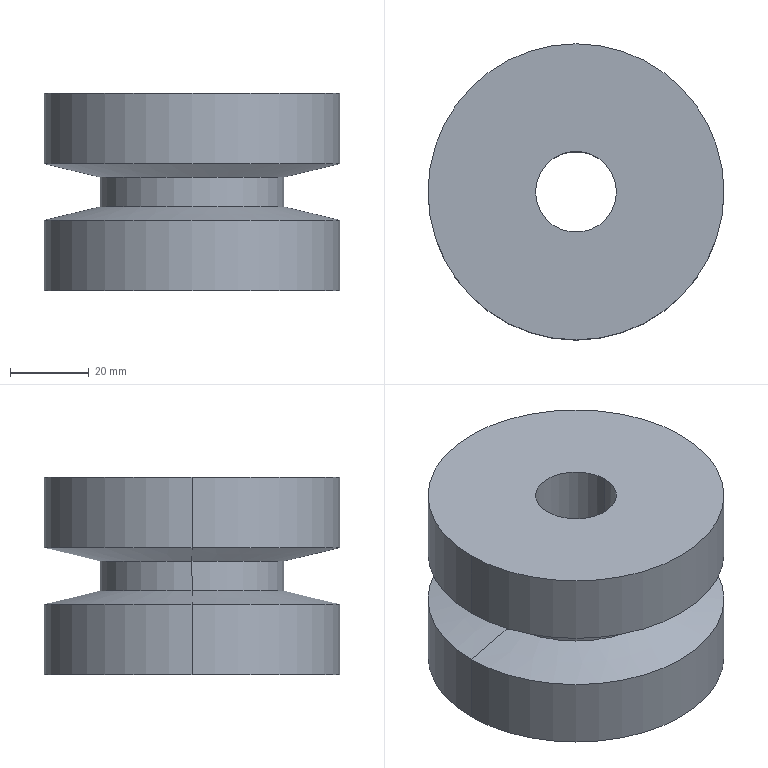Part | SolidWorks | features HoleWzd 2, Extrusion 1, RevCut 1 | 1 solid | 20 faces | box 75 x 75 x 50 mm | volume 173343 mm3 | cylinder 12 | cone 4 | plane 4 | commonest cylinder face diameters 4.2 x4 75 x4 20.5 x2 46.5 x2
STEP:
#1=CARTESIAN_POINT('',(10.25,0.,6.9));
#2=VERTEX_POINT('',#1);
#3=CARTESIAN_POINT('',(10.25,0.,11.1));
#4=VERTEX_POINT('',#3);
#5=CARTESIAN_POINT('',(10.25,0.,6.9));
#6=CARTESIAN_POINT('',(10.25,-0.1391,6.9));
#7=CARTESIAN_POINT('',(10.247,-0.2759,6.914));
#8=CARTESIAN_POINT('',(10.236,-0.5448,6.967));
#9=CARTESIAN_POINT('',(10.228,-0.6784,7.008));
#10=CARTESIAN_POINT('',(10.208,-0.9326,7.113));
#11=CARTESIAN_POINT('',(10.196,-1.053,7.178));
#12=CARTESIAN_POINT('',(10.17,-1.281,7.33));
#13=CARTESIAN_POINT('',(10.156,-1.389,7.419));
#14=CARTESIAN_POINT('',(10.114,-1.678,7.709));
#15=CARTESIAN_POINT('',(10.085,-1.835,7.942));
#16=CARTESIAN_POINT('',(10.055,-1.992,8.321));
#17=CARTESIAN_POINT('',(10.047,-2.032,8.454));
#18=CARTESIAN_POINT('',(10.035,-2.087,8.725));
#19=CARTESIAN_POINT('',(10.033,-2.1,8.862));
#20=CARTESIAN_POINT('',(10.033,-2.1,9.137));
#21=CARTESIAN_POINT('',(10.035,-2.086,9.276));
#22=CARTESIAN_POINT('',(10.047,-2.032,9.546));
#23=CARTESIAN_POINT('',(10.055,-1.993,9.677));
#24=CARTESIAN_POINT('',(10.085,-1.834,10.059));
#25=CARTESIAN_POINT('',(10.113,-1.68,10.29));
#26=CARTESIAN_POINT('',(10.156,-1.387,10.583));
#27=CARTESIAN_POINT('',(10.17,-1.282,10.669));
#28=CARTESIAN_POINT('',(10.196,-1.054,10.821));
#29=CARTESIAN_POINT('',(10.208,-0.9314,10.887));
#30=CARTESIAN_POINT('',(10.228,-0.6776,10.992));
#31=CARTESIAN_POINT('',(10.236,-0.5466,11.032));
#32=CARTESIAN_POINT('',(10.247,-0.2767,11.086));
#33=CARTESIAN_POINT('',(10.25,-0.1373,11.1));
#34=CARTESIAN_POINT('',(10.25,0.,11.1));
#35=B_SPLINE_CURVE_WITH_KNOTS('',3,(#5,#6,#7,#8,#9,#10,#11,#12,#13,#14,#15,#16,#17,#18,#19,#20,#21,#22,#23,#24,#25,#26,#27,#28,#29,#30,#31,#32,#33,#34),.UNSPECIFIED.,.F.,.F.,(4,2,2,2,2,2,2,2,2,2,2,2,2,2,4),(0.,0.0004114,0.0008229,0.001234,0.001646,0.002469,0.00288,0.003292,0.003703,0.004114,0.004937,0.005349,0.00576,0.006172,0.006583),.UNSPECIFIED.);
#36=EDGE_CURVE('',#2,#4,#35,.T.);
#37=ORIENTED_EDGE('',*,*,#36,.T.);
#38=CARTESIAN_POINT('',(32.5,0.,11.1));
#39=VERTEX_POINT('',#38);
#40=CARTESIAN_POINT('',(32.5,0.,11.1));
#41=DIRECTION('',(1.,0.,0.));
#42=VECTOR('',#41,1000.);
#43=LINE('',#40,#42);
#44=EDGE_CURVE('',#4,#39,#43,.T.);
#45=ORIENTED_EDGE('',*,*,#44,.T.);
#46=CARTESIAN_POINT('',(32.5,0.,6.9));
#47=VERTEX_POINT('',#46);
#48=CARTESIAN_POINT('',(32.5,0.,9.));
#49=DIRECTION('',(1.,0.,0.));
#50=DIRECTION('',(0.,0.,-1.));
#51=AXIS2_PLACEMENT_3D('',#48,#49,#50);
#52=CIRCLE('',#51,2.1);
#53=EDGE_CURVE('',#39,#47,#52,.T.);
#54=ORIENTED_EDGE('',*,*,#53,.T.);
#55=CARTESIAN_POINT('',(32.5,0.,6.9));
#56=DIRECTION('',(1.,0.,0.));
#57=VECTOR('',#56,1000.);
#58=LINE('',#55,#57);
#59=EDGE_CURVE('',#2,#47,#58,.T.);
#60=ORIENTED_EDGE('',*,*,#59,.F.);
#61=EDGE_LOOP('',(#37,#45,#54,#60));
#62=FACE_OUTER_BOUND('',#61,.T.);
#63=CARTESIAN_POINT('',(32.5,0.,9.));
#64=DIRECTION('',(1.,0.,0.));
#65=DIRECTION('',(0.,0.,-1.));
#66=AXIS2_PLACEMENT_3D('',#63,#64,#65);
#67=CYLINDRICAL_SURFACE('',#66,2.1);
#68=ADVANCED_FACE('',(#62),#67,.F.);
#69=CARTESIAN_POINT('',(0.,10.25,11.1));
#70=VERTEX_POINT('',#69);
#71=CARTESIAN_POINT('',(0.,10.25,6.9));
#72=VERTEX_POINT('',#71);
#73=CARTESIAN_POINT('',(0.,10.25,11.1));
#74=CARTESIAN_POINT('',(-0.1391,10.25,11.1));
#75=CARTESIAN_POINT('',(-0.2759,10.247,11.086));
#76=CARTESIAN_POINT('',(-0.5448,10.236,11.033));
#77=CARTESIAN_POINT('',(-0.6784,10.228,10.992));
#78=CARTESIAN_POINT('',(-0.9326,10.208,10.887));
#79=CARTESIAN_POINT('',(-1.053,10.196,10.822));
#80=CARTESIAN_POINT('',(-1.281,10.17,10.67));
#81=CARTESIAN_POINT('',(-1.389,10.156,10.581));
#82=CARTESIAN_POINT('',(-1.678,10.114,10.291));
#83=CARTESIAN_POINT('',(-1.835,10.085,10.058));
#84=CARTESIAN_POINT('',(-1.992,10.055,9.679));
#85=CARTESIAN_POINT('',(-2.032,10.047,9.546));
#86=CARTESIAN_POINT('',(-2.087,10.035,9.275));
#87=CARTESIAN_POINT('',(-2.1,10.033,9.138));
#88=CARTESIAN_POINT('',(-2.1,10.033,8.863));
#89=CARTESIAN_POINT('',(-2.086,10.035,8.724));
#90=CARTESIAN_POINT('',(-2.032,10.047,8.454));
#91=CARTESIAN_POINT('',(-1.993,10.055,8.323));
#92=CARTESIAN_POINT('',(-1.834,10.085,7.941));
#93=CARTESIAN_POINT('',(-1.68,10.113,7.71));
#94=CARTESIAN_POINT('',(-1.387,10.156,7.417));
#95=CARTESIAN_POINT('',(-1.282,10.17,7.331));
#96=CARTESIAN_POINT('',(-1.054,10.196,7.179));
#97=CARTESIAN_POINT('',(-0.9314,10.208,7.113));
#98=CARTESIAN_POINT('',(-0.6776,10.228,7.008));
#99=CARTESIAN_POINT('',(-0.5466,10.236,6.968));
#100=CARTESIAN_POINT('',(-0.2767,10.247,6.914));
#101=CARTESIAN_POINT('',(-0.1373,10.25,6.9));
#102=CARTESIAN_POINT('',(0.,10.25,6.9));
#103=B_SPLINE_CURVE_WITH_KNOTS('',3,(#73,#74,#75,#76,#77,#78,#79,#80,#81,#82,#83,#84,#85,#86,#87,#88,#89,#90,#91,#92,#93,#94,#95,#96,#97,#98,#99,#100,#101,#102),.UNSPECIFIED.,.F.,.F.,(4,2,2,2,2,2,2,2,2,2,2,2,2,2,4),(0.,0.0004114,0.0008229,0.001234,0.001646,0.002469,0.00288,0.003292,0.003703,0.004114,0.004937,0.005349,0.00576,0.006172,0.006583),.UNSPECIFIED.);
#104=EDGE_CURVE('',#70,#72,#103,.T.);
#105=ORIENTED_EDGE('',*,*,#104,.T.);
#106=CARTESIAN_POINT('',(0.,32.5,6.9));
#107=VERTEX_POINT('',#106);
#108=CARTESIAN_POINT('',(0.,32.5,6.9));
#109=DIRECTION('',(0.,1.,0.));
#110=VECTOR('',#109,1000.);
#111=LINE('',#108,#110);
#112=EDGE_CURVE('',#72,#107,#111,.T.);
#113=ORIENTED_EDGE('',*,*,#112,.T.);
#114=CARTESIAN_POINT('',(0.,32.5,11.1));
#115=VERTEX_POINT('',#114);
#116=CARTESIAN_POINT('',(0.,32.5,9.));
#117=DIRECTION('',(0.,1.,0.));
#118=DIRECTION('',(0.,0.,1.));
#119=AXIS2_PLACEMENT_3D('',#116,#117,#118);
#120=CIRCLE('',#119,2.1);
#121=EDGE_CURVE('',#107,#115,#120,.T.);
#122=ORIENTED_EDGE('',*,*,#121,.T.);
#123=CARTESIAN_POINT('',(0.,32.5,11.1));
#124=DIRECTION('',(0.,1.,0.));
#125=VECTOR('',#124,1000.);
#126=LINE('',#123,#125);
#127=EDGE_CURVE('',#70,#115,#126,.T.);
#128=ORIENTED_EDGE('',*,*,#127,.F.);
#129=EDGE_LOOP('',(#105,#113,#122,#128));
#130=FACE_OUTER_BOUND('',#129,.T.);
#131=CARTESIAN_POINT('',(0.,32.5,9.));
#132=DIRECTION('',(0.,1.,0.));
#133=DIRECTION('',(0.,0.,1.));
#134=AXIS2_PLACEMENT_3D('',#131,#132,#133);
#135=CYLINDRICAL_SURFACE('',#134,2.1);
#136=ADVANCED_FACE('',(#130),#135,.F.);
#137=CARTESIAN_POINT('',(-23.25,0.,28.75));
#138=VERTEX_POINT('',#137);
#139=CARTESIAN_POINT('',(23.25,0.,28.75));
#140=VERTEX_POINT('',#139);
#141=CARTESIAN_POINT('',(0.,0.,28.75));
#142=DIRECTION('',(0.,0.,-1.));
#143=DIRECTION('',(-1.,0.,0.));
#144=AXIS2_PLACEMENT_3D('',#141,#142,#143);
#145=CIRCLE('',#144,23.25);
#146=EDGE_CURVE('',#138,#140,#145,.T.);
#147=ORIENTED_EDGE('',*,*,#146,.T.);
#148=CARTESIAN_POINT('',(23.25,0.,21.25));
#149=VERTEX_POINT('',#148);
#150=CARTESIAN_POINT('',(23.25,0.,0.));
#151=DIRECTION('',(0.,0.,-1.));
#152=VECTOR('',#151,1000.);
#153=LINE('',#150,#152);
#154=EDGE_CURVE('',#140,#149,#153,.T.);
#155=ORIENTED_EDGE('',*,*,#154,.T.);
#156=CARTESIAN_POINT('',(-23.25,0.,21.25));
#157=VERTEX_POINT('',#156);
#158=CARTESIAN_POINT('',(0.,0.,21.25));
#159=DIRECTION('',(0.,0.,-1.));
#160=DIRECTION('',(-1.,0.,0.));
#161=AXIS2_PLACEMENT_3D('',#158,#159,#160);
#162=CIRCLE('',#161,23.25);
#163=EDGE_CURVE('',#157,#149,#162,.T.);
#164=ORIENTED_EDGE('',*,*,#163,.F.);
#165=CARTESIAN_POINT('',(-23.25,0.,0.));
#166=DIRECTION('',(0.,0.,-1.));
#167=VECTOR('',#166,1000.);
#168=LINE('',#165,#167);
#169=EDGE_CURVE('',#138,#157,#168,.T.);
#170=ORIENTED_EDGE('',*,*,#169,.F.);
#171=EDGE_LOOP('',(#147,#155,#164,#170));
#172=FACE_OUTER_BOUND('',#171,.T.);
#173=CARTESIAN_POINT('',(0.,0.,0.));
#174=DIRECTION('',(0.,0.,-1.));
#175=DIRECTION('',(-1.,0.,0.));
#176=AXIS2_PLACEMENT_3D('',#173,#174,#175);
#177=CYLINDRICAL_SURFACE('',#176,23.25);
#178=ADVANCED_FACE('',(#172),#177,.T.);
#179=ORIENTED_EDGE('',*,*,#146,.F.);
#180=CARTESIAN_POINT('',(-37.5,0.,32.171));
#181=VERTEX_POINT('',#180);
#182=CARTESIAN_POINT('',(-38.25,0.,32.351));
#183=DIRECTION('',(-0.9724,0.,0.2334));
#184=VECTOR('',#183,1000.);
#185=LINE('',#182,#184);
#186=EDGE_CURVE('',#138,#181,#185,.T.);
#187=ORIENTED_EDGE('',*,*,#186,.T.);
#188=CARTESIAN_POINT('',(37.5,0.,32.171));
#189=VERTEX_POINT('',#188);
#190=CARTESIAN_POINT('',(0.,0.,32.171));
#191=DIRECTION('',(0.,0.,1.));
#192=DIRECTION('',(1.,0.,0.));
#193=AXIS2_PLACEMENT_3D('',#190,#191,#192);
#194=CIRCLE('',#193,37.5);
#195=EDGE_CURVE('',#189,#181,#194,.T.);
#196=ORIENTED_EDGE('',*,*,#195,.F.);
#197=CARTESIAN_POINT('',(38.25,0.,32.351));
#198=DIRECTION('',(0.9724,0.,0.2334));
#199=VECTOR('',#198,1000.);
#200=LINE('',#197,#199);
#201=EDGE_CURVE('',#140,#189,#200,.T.);
#202=ORIENTED_EDGE('',*,*,#201,.F.);
#203=EDGE_LOOP('',(#179,#187,#196,#202));
#204=FACE_OUTER_BOUND('',#203,.T.);
#205=CARTESIAN_POINT('',(0.,0.,32.351));
#206=DIRECTION('',(0.,0.,1.));
#207=DIRECTION('',(1.,0.,0.));
#208=AXIS2_PLACEMENT_3D('',#205,#206,#207);
#209=CONICAL_SURFACE('',#208,38.25,1.335);
#210=ADVANCED_FACE('',(#204),#209,.T.);
#211=ORIENTED_EDGE('',*,*,#163,.T.);
#212=CARTESIAN_POINT('',(37.5,0.,17.829));
#213=VERTEX_POINT('',#212);
#214=CARTESIAN_POINT('',(23.25,0.,21.25));
#215=DIRECTION('',(0.9724,0.,-0.2334));
#216=VECTOR('',#215,1000.);
#217=LINE('',#214,#216);
#218=EDGE_CURVE('',#149,#213,#217,.T.);
#219=ORIENTED_EDGE('',*,*,#218,.T.);
#220=CARTESIAN_POINT('',(-37.5,0.,17.829));
#221=VERTEX_POINT('',#220);
#222=CARTESIAN_POINT('',(0.,0.,17.829));
#223=DIRECTION('',(0.,0.,-1.));
#224=DIRECTION('',(-1.,0.,0.));
#225=AXIS2_PLACEMENT_3D('',#222,#223,#224);
#226=CIRCLE('',#225,37.5);
#227=EDGE_CURVE('',#221,#213,#226,.T.);
#228=ORIENTED_EDGE('',*,*,#227,.F.);
#229=CARTESIAN_POINT('',(-23.25,0.,21.25));
#230=DIRECTION('',(-0.9724,0.,-0.2334));
#231=VECTOR('',#230,1000.);
#232=LINE('',#229,#231);
#233=EDGE_CURVE('',#157,#221,#232,.T.);
#234=ORIENTED_EDGE('',*,*,#233,.F.);
#235=EDGE_LOOP('',(#211,#219,#228,#234));
#236=FACE_OUTER_BOUND('',#235,.T.);
#237=CARTESIAN_POINT('',(0.,0.,21.25));
#238=DIRECTION('',(0.,0.,-1.));
#239=DIRECTION('',(-1.,0.,0.));
#240=AXIS2_PLACEMENT_3D('',#237,#238,#239);
#241=CONICAL_SURFACE('',#240,23.25,1.335);
#242=ADVANCED_FACE('',(#236),#241,.T.);
#243=CARTESIAN_POINT('',(-10.25,0.,50.));
#244=VERTEX_POINT('',#243);
#245=CARTESIAN_POINT('',(10.25,0.,50.));
#246=VERTEX_POINT('',#245);
#247=CARTESIAN_POINT('',(0.,0.,50.));
#248=DIRECTION('',(0.,0.,1.));
#249=DIRECTION('',(1.,0.,0.));
#250=AXIS2_PLACEMENT_3D('',#247,#248,#249);
#251=CIRCLE('',#250,10.25);
#252=EDGE_CURVE('',#244,#246,#251,.T.);
#253=ORIENTED_EDGE('',*,*,#252,.T.);
#254=CARTESIAN_POINT('',(10.25,0.,50.));
#255=DIRECTION('',(0.,0.,-1.));
#256=VECTOR('',#255,1000.);
#257=LINE('',#254,#256);
#258=EDGE_CURVE('',#246,#4,#257,.T.);
#259=ORIENTED_EDGE('',*,*,#258,.T.);
#260=ORIENTED_EDGE('',*,*,#36,.F.);
#261=CARTESIAN_POINT('',(10.25,0.,0.));
#262=VERTEX_POINT('',#261);
#263=CARTESIAN_POINT('',(10.25,0.,50.));
#264=DIRECTION('',(0.,0.,-1.));
#265=VECTOR('',#264,1000.);
#266=LINE('',#263,#265);
#267=EDGE_CURVE('',#2,#262,#266,.T.);
#268=ORIENTED_EDGE('',*,*,#267,.T.);
#269=CARTESIAN_POINT('',(-10.25,0.,0.));
#270=VERTEX_POINT('',#269);
#271=CARTESIAN_POINT('',(0.,0.,0.));
#272=DIRECTION('',(0.,0.,1.));
#273=DIRECTION('',(1.,0.,0.));
#274=AXIS2_PLACEMENT_3D('',#271,#272,#273);
#275=CIRCLE('',#274,10.25);
#276=EDGE_CURVE('',#270,#262,#275,.T.);
#277=ORIENTED_EDGE('',*,*,#276,.F.);
#278=CARTESIAN_POINT('',(-10.25,0.,50.));
#279=DIRECTION('',(0.,0.,-1.));
#280=VECTOR('',#279,1000.);
#281=LINE('',#278,#280);
#282=EDGE_CURVE('',#244,#270,#281,.T.);
#283=ORIENTED_EDGE('',*,*,#282,.F.);
#284=EDGE_LOOP('',(#253,#259,#260,#268,#277,#283));
#285=FACE_OUTER_BOUND('',#284,.T.);
#286=CARTESIAN_POINT('',(0.,0.,50.));
#287=DIRECTION('',(0.,0.,-1.));
#288=DIRECTION('',(-1.,0.,0.));
#289=AXIS2_PLACEMENT_3D('',#286,#287,#288);
#290=CYLINDRICAL_SURFACE('',#289,10.25);
#291=ADVANCED_FACE('',(#285),#290,.F.);
#292=CARTESIAN_POINT('',(37.5,0.,50.));
#293=VERTEX_POINT('',#292);
#294=CARTESIAN_POINT('',(-37.5,0.,50.));
#295=VERTEX_POINT('',#294);
#296=CARTESIAN_POINT('',(0.,0.,50.));
#297=DIRECTION('',(0.,0.,1.));
#298=DIRECTION('',(1.,0.,0.));
#299=AXIS2_PLACEMENT_3D('',#296,#297,#298);
#300=CIRCLE('',#299,37.5);
#301=EDGE_CURVE('',#293,#295,#300,.T.);
#302=ORIENTED_EDGE('',*,*,#301,.F.);
#303=CARTESIAN_POINT('',(37.5,0.,50.));
#304=DIRECTION('',(0.,0.,-1.));
#305=VECTOR('',#304,1000.);
#306=LINE('',#303,#305);
#307=EDGE_CURVE('',#293,#189,#306,.T.);
#308=ORIENTED_EDGE('',*,*,#307,.T.);
#309=ORIENTED_EDGE('',*,*,#195,.T.);
#310=CARTESIAN_POINT('',(-37.5,0.,50.));
#311=DIRECTION('',(0.,0.,-1.));
#312=VECTOR('',#311,1000.);
#313=LINE('',#310,#312);
#314=EDGE_CURVE('',#295,#181,#313,.T.);
#315=ORIENTED_EDGE('',*,*,#314,.F.);
#316=EDGE_LOOP('',(#302,#308,#309,#315));
#317=FACE_OUTER_BOUND('',#316,.T.);
#318=CARTESIAN_POINT('',(0.,0.,50.));
#319=DIRECTION('',(0.,0.,-1.));
#320=DIRECTION('',(-1.,0.,0.));
#321=AXIS2_PLACEMENT_3D('',#318,#319,#320);
#322=CYLINDRICAL_SURFACE('',#321,37.5);
#323=ADVANCED_FACE('',(#317),#322,.T.);
#324=ORIENTED_EDGE('',*,*,#227,.T.);
#325=CARTESIAN_POINT('',(37.5,0.,0.));
#326=VERTEX_POINT('',#325);
#327=CARTESIAN_POINT('',(37.5,0.,50.));
#328=DIRECTION('',(0.,0.,-1.));
#329=VECTOR('',#328,1000.);
#330=LINE('',#327,#329);
#331=EDGE_CURVE('',#213,#326,#330,.T.);
#332=ORIENTED_EDGE('',*,*,#331,.T.);
#333=CARTESIAN_POINT('',(-37.5,0.,0.));
#334=VERTEX_POINT('',#333);
#335=CARTESIAN_POINT('',(0.,0.,0.));
#336=DIRECTION('',(0.,0.,1.));
#337=DIRECTION('',(1.,0.,0.));
#338=AXIS2_PLACEMENT_3D('',#335,#336,#337);
#339=CIRCLE('',#338,37.5);
#340=EDGE_CURVE('',#326,#334,#339,.T.);
#341=ORIENTED_EDGE('',*,*,#340,.T.);
#342=CARTESIAN_POINT('',(-37.5,0.,50.));
#343=DIRECTION('',(0.,0.,-1.));
#344=VECTOR('',#343,1000.);
#345=LINE('',#342,#344);
#346=EDGE_CURVE('',#221,#334,#345,.T.);
#347=ORIENTED_EDGE('',*,*,#346,.F.);
#348=EDGE_LOOP('',(#324,#332,#341,#347));
#349=FACE_OUTER_BOUND('',#348,.T.);
#350=CARTESIAN_POINT('',(0.,0.,50.));
#351=DIRECTION('',(0.,0.,-1.));
#352=DIRECTION('',(-1.,0.,0.));
#353=AXIS2_PLACEMENT_3D('',#350,#351,#352);
#354=CYLINDRICAL_SURFACE('',#353,37.5);
#355=ADVANCED_FACE('',(#349),#354,.T.);
#356=ORIENTED_EDGE('',*,*,#331,.F.);
#357=CARTESIAN_POINT('',(0.,0.,17.829));
#358=DIRECTION('',(0.,0.,-1.));
#359=DIRECTION('',(-1.,0.,0.));
#360=AXIS2_PLACEMENT_3D('',#357,#358,#359);
#361=CIRCLE('',#360,37.5);
#362=EDGE_CURVE('',#213,#221,#361,.T.);
#363=ORIENTED_EDGE('',*,*,#362,.T.);
#364=ORIENTED_EDGE('',*,*,#346,.T.);
#365=CARTESIAN_POINT('',(0.,0.,0.));
#366=DIRECTION('',(0.,0.,1.));
#367=DIRECTION('',(1.,0.,0.));
#368=AXIS2_PLACEMENT_3D('',#365,#366,#367);
#369=CIRCLE('',#368,37.5);
#370=EDGE_CURVE('',#334,#326,#369,.T.);
#371=ORIENTED_EDGE('',*,*,#370,.T.);
#372=EDGE_LOOP('',(#356,#363,#364,#371));
#373=FACE_OUTER_BOUND('',#372,.T.);
#374=CARTESIAN_POINT('',(0.,0.,50.));
#375=DIRECTION('',(0.,0.,-1.));
#376=DIRECTION('',(-1.,0.,0.));
#377=AXIS2_PLACEMENT_3D('',#374,#375,#376);
#378=CYLINDRICAL_SURFACE('',#377,37.5);
#379=ADVANCED_FACE('',(#373),#378,.T.);
#380=CARTESIAN_POINT('',(0.,0.,50.));
#381=DIRECTION('',(0.,0.,1.));
#382=DIRECTION('',(1.,0.,0.));
#383=AXIS2_PLACEMENT_3D('',#380,#381,#382);
#384=CIRCLE('',#383,37.5);
#385=EDGE_CURVE('',#295,#293,#384,.T.);
#386=ORIENTED_EDGE('',*,*,#385,.T.);
#387=ORIENTED_EDGE('',*,*,#301,.T.);
#388=EDGE_LOOP('',(#386,#387));
#389=FACE_OUTER_BOUND('',#388,.T.);
#390=ORIENTED_EDGE('',*,*,#252,.F.);
#391=CARTESIAN_POINT('',(0.,0.,50.));
#392=DIRECTION('',(0.,0.,1.));
#393=DIRECTION('',(1.,0.,0.));
#394=AXIS2_PLACEMENT_3D('',#391,#392,#393);
#395=CIRCLE('',#394,10.25);
#396=EDGE_CURVE('',#246,#244,#395,.T.);
#397=ORIENTED_EDGE('',*,*,#396,.F.);
#398=EDGE_LOOP('',(#390,#397));
#399=FACE_BOUND('',#398,.T.);
#400=CARTESIAN_POINT('',(0.,0.,50.));
#401=DIRECTION('',(0.,0.,1.));
#402=DIRECTION('',(1.,0.,0.));
#403=AXIS2_PLACEMENT_3D('',#400,#401,#402);
#404=PLANE('',#403);
#405=ADVANCED_FACE('',(#389,#399),#404,.T.);
#406=ORIENTED_EDGE('',*,*,#370,.F.);
#407=ORIENTED_EDGE('',*,*,#340,.F.);
#408=EDGE_LOOP('',(#406,#407));
#409=FACE_OUTER_BOUND('',#408,.T.);
#410=ORIENTED_EDGE('',*,*,#276,.T.);
#411=CARTESIAN_POINT('',(0.,0.,0.));
#412=DIRECTION('',(0.,0.,1.));
#413=DIRECTION('',(1.,0.,0.));
#414=AXIS2_PLACEMENT_3D('',#411,#412,#413);
#415=CIRCLE('',#414,10.25);
#416=EDGE_CURVE('',#262,#270,#415,.T.);
#417=ORIENTED_EDGE('',*,*,#416,.T.);
#418=EDGE_LOOP('',(#410,#417));
#419=FACE_BOUND('',#418,.T.);
#420=CARTESIAN_POINT('',(0.,0.,0.));
#421=DIRECTION('',(0.,0.,1.));
#422=DIRECTION('',(1.,0.,0.));
#423=AXIS2_PLACEMENT_3D('',#420,#421,#422);
#424=PLANE('',#423);
#425=ADVANCED_FACE('',(#409,#419),#424,.F.);
#426=ORIENTED_EDGE('',*,*,#307,.F.);
#427=ORIENTED_EDGE('',*,*,#385,.F.);
#428=ORIENTED_EDGE('',*,*,#314,.T.);
#429=CARTESIAN_POINT('',(0.,0.,32.171));
#430=DIRECTION('',(0.,0.,1.));
#431=DIRECTION('',(1.,0.,0.));
#432=AXIS2_PLACEMENT_3D('',#429,#430,#431);
#433=CIRCLE('',#432,37.5);
#434=EDGE_CURVE('',#181,#189,#433,.T.);
#435=ORIENTED_EDGE('',*,*,#434,.T.);
#436=EDGE_LOOP('',(#426,#427,#428,#435));
#437=FACE_OUTER_BOUND('',#436,.T.);
#438=CARTESIAN_POINT('',(0.,0.,50.));
#439=DIRECTION('',(0.,0.,-1.));
#440=DIRECTION('',(-1.,0.,0.));
#441=AXIS2_PLACEMENT_3D('',#438,#439,#440);
#442=CYLINDRICAL_SURFACE('',#441,37.5);
#443=ADVANCED_FACE('',(#437),#442,.T.);
#444=ORIENTED_EDGE('',*,*,#258,.F.);
#445=ORIENTED_EDGE('',*,*,#396,.T.);
#446=ORIENTED_EDGE('',*,*,#282,.T.);
#447=ORIENTED_EDGE('',*,*,#416,.F.);
#448=ORIENTED_EDGE('',*,*,#267,.F.);
#449=CARTESIAN_POINT('',(10.25,0.,11.1));
#450=CARTESIAN_POINT('',(10.25,0.2744,11.1));
#451=CARTESIAN_POINT('',(10.238,0.5514,11.045));
#452=CARTESIAN_POINT('',(10.208,0.9307,10.887));
#453=CARTESIAN_POINT('',(10.196,1.053,10.822));
#454=CARTESIAN_POINT('',(10.17,1.282,10.669));
#455=CARTESIAN_POINT('',(10.156,1.387,10.582));
#456=CARTESIAN_POINT('',(10.128,1.581,10.389));
#457=CARTESIAN_POINT('',(10.113,1.669,10.281));
#458=CARTESIAN_POINT('',(10.087,1.821,10.054));
#459=CARTESIAN_POINT('',(10.075,1.886,9.934));
#460=CARTESIAN_POINT('',(10.045,2.045,9.551));
#461=CARTESIAN_POINT('',(10.033,2.1,9.278));
#462=CARTESIAN_POINT('',(10.033,2.1,8.862));
#463=CARTESIAN_POINT('',(10.035,2.087,8.726));
#464=CARTESIAN_POINT('',(10.046,2.033,8.457));
#465=CARTESIAN_POINT('',(10.055,1.993,8.323));
#466=CARTESIAN_POINT('',(10.075,1.887,8.069));
#467=CARTESIAN_POINT('',(10.087,1.823,7.949));
#468=CARTESIAN_POINT('',(10.113,1.67,7.72));
#469=CARTESIAN_POINT('',(10.128,1.582,7.613));
#470=CARTESIAN_POINT('',(10.17,1.293,7.323));
#471=CARTESIAN_POINT('',(10.198,1.059,7.166));
#472=CARTESIAN_POINT('',(10.228,0.6807,7.009));
#473=CARTESIAN_POINT('',(10.236,0.5474,6.968));
#474=CARTESIAN_POINT('',(10.247,0.2764,6.914));
#475=CARTESIAN_POINT('',(10.25,0.1391,6.9));
#476=CARTESIAN_POINT('',(10.25,0.,6.9));
#477=B_SPLINE_CURVE_WITH_KNOTS('',3,(#449,#450,#451,#452,#453,#454,#455,#456,#457,#458,#459,#460,#461,#462,#463,#464,#465,#466,#467,#468,#469,#470,#471,#472,#473,#474,#475,#476),.UNSPECIFIED.,.F.,.F.,(4,2,2,2,2,2,2,2,2,2,2,2,2,4),(0.006583,0.007406,0.007817,0.008228,0.00864,0.009051,0.009874,0.01029,0.0107,0.01111,0.01152,0.01234,0.01275,0.01316),.UNSPECIFIED.);
#478=EDGE_CURVE('',#4,#2,#477,.T.);
#479=ORIENTED_EDGE('',*,*,#478,.F.);
#480=EDGE_LOOP('',(#444,#445,#446,#447,#448,#479));
#481=FACE_OUTER_BOUND('',#480,.T.);
#482=ORIENTED_EDGE('',*,*,#104,.F.);
#483=CARTESIAN_POINT('',(0.,10.25,6.9));
#484=CARTESIAN_POINT('',(0.2744,10.25,6.9));
#485=CARTESIAN_POINT('',(0.5514,10.238,6.955));
#486=CARTESIAN_POINT('',(0.9307,10.208,7.113));
#487=CARTESIAN_POINT('',(1.053,10.196,7.178));
#488=CARTESIAN_POINT('',(1.282,10.17,7.331));
#489=CARTESIAN_POINT('',(1.387,10.156,7.418));
#490=CARTESIAN_POINT('',(1.581,10.128,7.611));
#491=CARTESIAN_POINT('',(1.669,10.113,7.719));
#492=CARTESIAN_POINT('',(1.821,10.087,7.946));
#493=CARTESIAN_POINT('',(1.886,10.075,8.066));
#494=CARTESIAN_POINT('',(2.045,10.045,8.449));
#495=CARTESIAN_POINT('',(2.1,10.033,8.722));
#496=CARTESIAN_POINT('',(2.1,10.033,9.138));
#497=CARTESIAN_POINT('',(2.087,10.035,9.274));
#498=CARTESIAN_POINT('',(2.033,10.046,9.543));
#499=CARTESIAN_POINT('',(1.993,10.055,9.677));
#500=CARTESIAN_POINT('',(1.887,10.075,9.931));
#501=CARTESIAN_POINT('',(1.823,10.087,10.051));
#502=CARTESIAN_POINT('',(1.67,10.113,10.28));
#503=CARTESIAN_POINT('',(1.582,10.128,10.387));
#504=CARTESIAN_POINT('',(1.293,10.17,10.677));
#505=CARTESIAN_POINT('',(1.059,10.198,10.834));
#506=CARTESIAN_POINT('',(0.6807,10.228,10.991));
#507=CARTESIAN_POINT('',(0.5474,10.236,11.032));
#508=CARTESIAN_POINT('',(0.2764,10.247,11.086));
#509=CARTESIAN_POINT('',(0.1391,10.25,11.1));
#510=CARTESIAN_POINT('',(0.,10.25,11.1));
#511=B_SPLINE_CURVE_WITH_KNOTS('',3,(#483,#484,#485,#486,#487,#488,#489,#490,#491,#492,#493,#494,#495,#496,#497,#498,#499,#500,#501,#502,#503,#504,#505,#506,#507,#508,#509,#510),.UNSPECIFIED.,.F.,.F.,(4,2,2,2,2,2,2,2,2,2,2,2,2,4),(0.006583,0.007406,0.007817,0.008228,0.00864,0.009051,0.009874,0.01029,0.0107,0.01111,0.01152,0.01234,0.01275,0.01316),.UNSPECIFIED.);
#512=EDGE_CURVE('',#72,#70,#511,.T.);
#513=ORIENTED_EDGE('',*,*,#512,.F.);
#514=EDGE_LOOP('',(#482,#513));
#515=FACE_BOUND('',#514,.T.);
#516=CARTESIAN_POINT('',(0.,0.,50.));
#517=DIRECTION('',(0.,0.,-1.));
#518=DIRECTION('',(-1.,0.,0.));
#519=AXIS2_PLACEMENT_3D('',#516,#517,#518);
#520=CYLINDRICAL_SURFACE('',#519,10.25);
#521=ADVANCED_FACE('',(#481,#515),#520,.F.);
#522=ORIENTED_EDGE('',*,*,#218,.F.);
#523=CARTESIAN_POINT('',(0.,0.,21.25));
#524=DIRECTION('',(0.,0.,-1.));
#525=DIRECTION('',(-1.,0.,0.));
#526=AXIS2_PLACEMENT_3D('',#523,#524,#525);
#527=CIRCLE('',#526,23.25);
#528=EDGE_CURVE('',#149,#157,#527,.T.);
#529=ORIENTED_EDGE('',*,*,#528,.T.);
#530=ORIENTED_EDGE('',*,*,#233,.T.);
#531=ORIENTED_EDGE('',*,*,#362,.F.);
#532=EDGE_LOOP('',(#522,#529,#530,#531));
#533=FACE_OUTER_BOUND('',#532,.T.);
#534=CARTESIAN_POINT('',(0.,0.,21.25));
#535=DIRECTION('',(0.,0.,-1.));
#536=DIRECTION('',(-1.,0.,0.));
#537=AXIS2_PLACEMENT_3D('',#534,#535,#536);
#538=CONICAL_SURFACE('',#537,23.25,1.335);
#539=ADVANCED_FACE('',(#533),#538,.T.);
#540=ORIENTED_EDGE('',*,*,#186,.F.);
#541=CARTESIAN_POINT('',(0.,0.,28.75));
#542=DIRECTION('',(0.,0.,-1.));
#543=DIRECTION('',(-1.,0.,0.));
#544=AXIS2_PLACEMENT_3D('',#541,#542,#543);
#545=CIRCLE('',#544,23.25);
#546=EDGE_CURVE('',#140,#138,#545,.T.);
#547=ORIENTED_EDGE('',*,*,#546,.F.);
#548=ORIENTED_EDGE('',*,*,#201,.T.);
#549=ORIENTED_EDGE('',*,*,#434,.F.);
#550=EDGE_LOOP('',(#540,#547,#548,#549));
#551=FACE_OUTER_BOUND('',#550,.T.);
#552=CARTESIAN_POINT('',(0.,0.,32.351));
#553=DIRECTION('',(0.,0.,1.));
#554=DIRECTION('',(1.,0.,0.));
#555=AXIS2_PLACEMENT_3D('',#552,#553,#554);
#556=CONICAL_SURFACE('',#555,38.25,1.335);
#557=ADVANCED_FACE('',(#551),#556,.T.);
#558=ORIENTED_EDGE('',*,*,#154,.F.);
#559=ORIENTED_EDGE('',*,*,#546,.T.);
#560=ORIENTED_EDGE('',*,*,#169,.T.);
#561=ORIENTED_EDGE('',*,*,#528,.F.);
#562=EDGE_LOOP('',(#558,#559,#560,#561));
#563=FACE_OUTER_BOUND('',#562,.T.);
#564=CARTESIAN_POINT('',(0.,0.,0.));
#565=DIRECTION('',(0.,0.,-1.));
#566=DIRECTION('',(-1.,0.,0.));
#567=AXIS2_PLACEMENT_3D('',#564,#565,#566);
#568=CYLINDRICAL_SURFACE('',#567,23.25);
#569=ADVANCED_FACE('',(#563),#568,.T.);
#570=CARTESIAN_POINT('',(0.,32.5,9.));
#571=DIRECTION('',(0.,1.,0.));
#572=DIRECTION('',(0.,0.,1.));
#573=AXIS2_PLACEMENT_3D('',#570,#571,#572);
#574=CIRCLE('',#573,2.1);
#575=EDGE_CURVE('',#115,#107,#574,.T.);
#576=ORIENTED_EDGE('',*,*,#575,.F.);
#577=ORIENTED_EDGE('',*,*,#121,.F.);
#578=EDGE_LOOP('',(#576,#577));
#579=FACE_OUTER_BOUND('',#578,.T.);
#580=CARTESIAN_POINT('',(2.1,32.5,9.));
#581=DIRECTION('',(0.,1.,0.));
#582=DIRECTION('',(0.,0.,1.));
#583=AXIS2_PLACEMENT_3D('',#580,#581,#582);
#584=PLANE('',#583);
#585=ADVANCED_FACE('',(#579),#584,.F.);
#586=ORIENTED_EDGE('',*,*,#112,.F.);
#587=ORIENTED_EDGE('',*,*,#512,.T.);
#588=ORIENTED_EDGE('',*,*,#127,.T.);
#589=ORIENTED_EDGE('',*,*,#575,.T.);
#590=EDGE_LOOP('',(#586,#587,#588,#589));
#591=FACE_OUTER_BOUND('',#590,.T.);
#592=CARTESIAN_POINT('',(0.,32.5,9.));
#593=DIRECTION('',(0.,1.,0.));
#594=DIRECTION('',(0.,0.,1.));
#595=AXIS2_PLACEMENT_3D('',#592,#593,#594);
#596=CYLINDRICAL_SURFACE('',#595,2.1);
#597=ADVANCED_FACE('',(#591),#596,.F.);
#598=CARTESIAN_POINT('',(32.5,0.,9.));
#599=DIRECTION('',(1.,0.,0.));
#600=DIRECTION('',(0.,0.,-1.));
#601=AXIS2_PLACEMENT_3D('',#598,#599,#600);
#602=CIRCLE('',#601,2.1);
#603=EDGE_CURVE('',#47,#39,#602,.T.);
#604=ORIENTED_EDGE('',*,*,#603,.F.);
#605=ORIENTED_EDGE('',*,*,#53,.F.);
#606=EDGE_LOOP('',(#604,#605));
#607=FACE_OUTER_BOUND('',#606,.T.);
#608=CARTESIAN_POINT('',(32.5,2.1,9.));
#609=DIRECTION('',(1.,0.,0.));
#610=DIRECTION('',(0.,0.,-1.));
#611=AXIS2_PLACEMENT_3D('',#608,#609,#610);
#612=PLANE('',#611);
#613=ADVANCED_FACE('',(#607),#612,.F.);
#614=ORIENTED_EDGE('',*,*,#44,.F.);
#615=ORIENTED_EDGE('',*,*,#478,.T.);
#616=ORIENTED_EDGE('',*,*,#59,.T.);
#617=ORIENTED_EDGE('',*,*,#603,.T.);
#618=EDGE_LOOP('',(#614,#615,#616,#617));
#619=FACE_OUTER_BOUND('',#618,.T.);
#620=CARTESIAN_POINT('',(32.5,0.,9.));
#621=DIRECTION('',(1.,0.,0.));
#622=DIRECTION('',(0.,0.,-1.));
#623=AXIS2_PLACEMENT_3D('',#620,#621,#622);
#624=CYLINDRICAL_SURFACE('',#623,2.1);
#625=ADVANCED_FACE('',(#619),#624,.F.);
#626=CLOSED_SHELL('',(#68,#136,#178,#210,#242,#291,#323,#355,#379,#405,#425,#443,#521,#539,#557,#569,#585,#597,#613,#625));
#627=MANIFOLD_SOLID_BREP('',#626);
#628=CARTESIAN_POINT('',(0.,0.,0.));
#629=DIRECTION('',(0.,0.,1.));
#630=DIRECTION('',(1.,0.,0.));
#631=AXIS2_PLACEMENT_3D('',#628,#629,#630);
#632=(LENGTH_UNIT()NAMED_UNIT(*)SI_UNIT(.MILLI.,.METRE.));
#633=UNCERTAINTY_MEASURE_WITH_UNIT(LENGTH_MEASURE(0.00001),#632,'','');
#634=(NAMED_UNIT(*)PLANE_ANGLE_UNIT()SI_UNIT($,.RADIAN.));
#635=(NAMED_UNIT(*)SI_UNIT($,.STERADIAN.)SOLID_ANGLE_UNIT());
#636=(GEOMETRIC_REPRESENTATION_CONTEXT(3)GLOBAL_UNCERTAINTY_ASSIGNED_CONTEXT((#633))GLOBAL_UNIT_ASSIGNED_CONTEXT((#632,#634,#635))REPRESENTATION_CONTEXT('',''));
#637=ADVANCED_BREP_SHAPE_REPRESENTATION('',(#627,#631),#636);